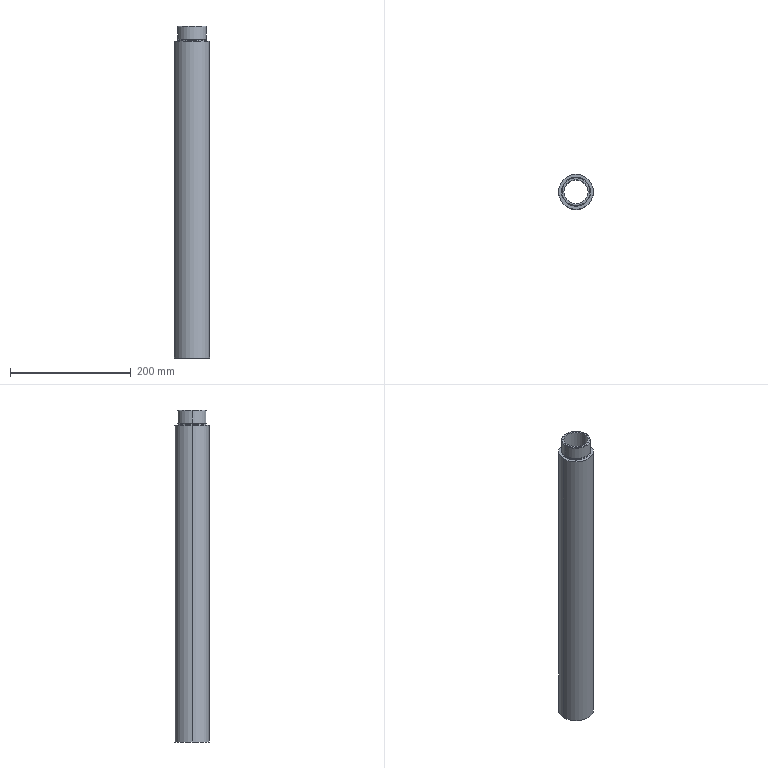Part | SolidWorks | features ICE 3, Chamfer 1, Extrusion 1, Fillet 1 | 1 solid | 18 faces | box 58 x 58 x 550 mm | volume 740682 mm3 | cylinder 8 | torus 4 | plane 4 | cone 2 | commonest cylinder face diameters 40 x2 45.8 x2 48 x2 58 x2
STEP:
#1=CARTESIAN_POINT('',(-23.9,0.,528.));
#2=VERTEX_POINT('',#1);
#3=CARTESIAN_POINT('',(23.9,0.,528.));
#4=VERTEX_POINT('',#3);
#5=CARTESIAN_POINT('',(0.,0.,528.));
#6=DIRECTION('',(0.,0.,1.));
#7=DIRECTION('',(1.,0.,0.));
#8=AXIS2_PLACEMENT_3D('',#5,#6,#7);
#9=CIRCLE('',#8,23.9);
#10=EDGE_CURVE('',#2,#4,#9,.T.);
#11=ORIENTED_EDGE('',*,*,#10,.F.);
#12=CARTESIAN_POINT('',(-22.9,0.,527.));
#13=VERTEX_POINT('',#12);
#14=CARTESIAN_POINT('',(-23.9,0.,527.));
#15=DIRECTION('',(0.,1.,0.));
#16=DIRECTION('',(-1.,0.,0.));
#17=AXIS2_PLACEMENT_3D('',#14,#15,#16);
#18=CIRCLE('',#17,1.);
#19=EDGE_CURVE('',#2,#13,#18,.T.);
#20=ORIENTED_EDGE('',*,*,#19,.T.);
#21=CARTESIAN_POINT('',(22.9,0.,527.));
#22=VERTEX_POINT('',#21);
#23=CARTESIAN_POINT('',(0.,0.,527.));
#24=DIRECTION('',(0.,0.,-1.));
#25=DIRECTION('',(1.,0.,0.));
#26=AXIS2_PLACEMENT_3D('',#23,#24,#25);
#27=CIRCLE('',#26,22.9);
#28=EDGE_CURVE('',#22,#13,#27,.T.);
#29=ORIENTED_EDGE('',*,*,#28,.F.);
#30=CARTESIAN_POINT('',(23.9,0.,527.));
#31=DIRECTION('',(0.,-1.,0.));
#32=DIRECTION('',(0.,0.,-1.));
#33=AXIS2_PLACEMENT_3D('',#30,#31,#32);
#34=CIRCLE('',#33,1.);
#35=EDGE_CURVE('',#4,#22,#34,.T.);
#36=ORIENTED_EDGE('',*,*,#35,.F.);
#37=EDGE_LOOP('',(#11,#20,#29,#36));
#38=FACE_OUTER_BOUND('',#37,.T.);
#39=CARTESIAN_POINT('',(0.,0.,527.));
#40=DIRECTION('',(0.,0.,1.));
#41=DIRECTION('',(1.,0.,0.));
#42=AXIS2_PLACEMENT_3D('',#39,#40,#41);
#43=TOROIDAL_SURFACE('',#42,23.9,1.);
#44=ADVANCED_FACE('',(#38),#43,.F.);
#45=CARTESIAN_POINT('',(-22.9,0.,526.));
#46=VERTEX_POINT('',#45);
#47=CARTESIAN_POINT('',(22.9,0.,526.));
#48=VERTEX_POINT('',#47);
#49=CARTESIAN_POINT('',(0.,0.,526.));
#50=DIRECTION('',(0.,0.,1.));
#51=DIRECTION('',(1.,0.,0.));
#52=AXIS2_PLACEMENT_3D('',#49,#50,#51);
#53=CIRCLE('',#52,22.9);
#54=EDGE_CURVE('',#46,#48,#53,.T.);
#55=ORIENTED_EDGE('',*,*,#54,.F.);
#56=CARTESIAN_POINT('',(-23.9,0.,525.));
#57=VERTEX_POINT('',#56);
#58=CARTESIAN_POINT('',(-23.9,0.,526.));
#59=DIRECTION('',(0.,1.,0.));
#60=DIRECTION('',(-1.,0.,0.));
#61=AXIS2_PLACEMENT_3D('',#58,#59,#60);
#62=CIRCLE('',#61,1.);
#63=EDGE_CURVE('',#46,#57,#62,.T.);
#64=ORIENTED_EDGE('',*,*,#63,.T.);
#65=CARTESIAN_POINT('',(23.9,0.,525.));
#66=VERTEX_POINT('',#65);
#67=CARTESIAN_POINT('',(0.,0.,525.));
#68=DIRECTION('',(0.,0.,-1.));
#69=DIRECTION('',(1.,0.,0.));
#70=AXIS2_PLACEMENT_3D('',#67,#68,#69);
#71=CIRCLE('',#70,23.9);
#72=EDGE_CURVE('',#66,#57,#71,.T.);
#73=ORIENTED_EDGE('',*,*,#72,.F.);
#74=CARTESIAN_POINT('',(23.9,0.,526.));
#75=DIRECTION('',(0.,-1.,0.));
#76=DIRECTION('',(0.,0.,-1.));
#77=AXIS2_PLACEMENT_3D('',#74,#75,#76);
#78=CIRCLE('',#77,1.);
#79=EDGE_CURVE('',#48,#66,#78,.T.);
#80=ORIENTED_EDGE('',*,*,#79,.F.);
#81=EDGE_LOOP('',(#55,#64,#73,#80));
#82=FACE_OUTER_BOUND('',#81,.T.);
#83=CARTESIAN_POINT('',(0.,0.,526.));
#84=DIRECTION('',(0.,0.,1.));
#85=DIRECTION('',(1.,0.,0.));
#86=AXIS2_PLACEMENT_3D('',#83,#84,#85);
#87=TOROIDAL_SURFACE('',#86,23.9,1.);
#88=ADVANCED_FACE('',(#82),#87,.F.);
#89=CARTESIAN_POINT('',(0.,0.,527.));
#90=DIRECTION('',(0.,0.,-1.));
#91=DIRECTION('',(1.,0.,0.));
#92=AXIS2_PLACEMENT_3D('',#89,#90,#91);
#93=CIRCLE('',#92,22.9);
#94=EDGE_CURVE('',#13,#22,#93,.T.);
#95=ORIENTED_EDGE('',*,*,#94,.T.);
#96=CARTESIAN_POINT('',(22.9,0.,528.));
#97=DIRECTION('',(0.,0.,-1.));
#98=VECTOR('',#97,1000.);
#99=LINE('',#96,#98);
#100=EDGE_CURVE('',#22,#48,#99,.T.);
#101=ORIENTED_EDGE('',*,*,#100,.T.);
#102=CARTESIAN_POINT('',(0.,0.,526.));
#103=DIRECTION('',(0.,0.,1.));
#104=DIRECTION('',(1.,0.,0.));
#105=AXIS2_PLACEMENT_3D('',#102,#103,#104);
#106=CIRCLE('',#105,22.9);
#107=EDGE_CURVE('',#48,#46,#106,.T.);
#108=ORIENTED_EDGE('',*,*,#107,.T.);
#109=CARTESIAN_POINT('',(-22.9,0.,528.));
#110=DIRECTION('',(0.,0.,-1.));
#111=VECTOR('',#110,1000.);
#112=LINE('',#109,#111);
#113=EDGE_CURVE('',#13,#46,#112,.T.);
#114=ORIENTED_EDGE('',*,*,#113,.F.);
#115=EDGE_LOOP('',(#95,#101,#108,#114));
#116=FACE_OUTER_BOUND('',#115,.T.);
#117=CARTESIAN_POINT('',(0.,0.,528.));
#118=DIRECTION('',(0.,0.,-1.));
#119=DIRECTION('',(-1.,0.,0.));
#120=AXIS2_PLACEMENT_3D('',#117,#118,#119);
#121=CYLINDRICAL_SURFACE('',#120,22.9);
#122=ADVANCED_FACE('',(#116),#121,.T.);
#123=CARTESIAN_POINT('',(23.,0.,550.));
#124=VERTEX_POINT('',#123);
#125=CARTESIAN_POINT('',(-23.,0.,550.));
#126=VERTEX_POINT('',#125);
#127=CARTESIAN_POINT('',(0.,0.,550.));
#128=DIRECTION('',(0.,0.,1.));
#129=DIRECTION('',(1.,0.,0.));
#130=AXIS2_PLACEMENT_3D('',#127,#128,#129);
#131=CIRCLE('',#130,23.);
#132=EDGE_CURVE('',#124,#126,#131,.T.);
#133=ORIENTED_EDGE('',*,*,#132,.F.);
#134=CARTESIAN_POINT('',(24.,0.,549.));
#135=VERTEX_POINT('',#134);
#136=CARTESIAN_POINT('',(23.,0.,550.));
#137=DIRECTION('',(0.7071,0.,-0.7071));
#138=VECTOR('',#137,1000.);
#139=LINE('',#136,#138);
#140=EDGE_CURVE('',#124,#135,#139,.T.);
#141=ORIENTED_EDGE('',*,*,#140,.T.);
#142=CARTESIAN_POINT('',(-24.,0.,549.));
#143=VERTEX_POINT('',#142);
#144=CARTESIAN_POINT('',(0.,0.,549.));
#145=DIRECTION('',(0.,0.,-1.));
#146=DIRECTION('',(1.,0.,0.));
#147=AXIS2_PLACEMENT_3D('',#144,#145,#146);
#148=CIRCLE('',#147,24.);
#149=EDGE_CURVE('',#143,#135,#148,.T.);
#150=ORIENTED_EDGE('',*,*,#149,.F.);
#151=CARTESIAN_POINT('',(-23.,0.,550.));
#152=DIRECTION('',(-0.7071,0.,-0.7071));
#153=VECTOR('',#152,1000.);
#154=LINE('',#151,#153);
#155=EDGE_CURVE('',#126,#143,#154,.T.);
#156=ORIENTED_EDGE('',*,*,#155,.F.);
#157=EDGE_LOOP('',(#133,#141,#150,#156));
#158=FACE_OUTER_BOUND('',#157,.T.);
#159=CARTESIAN_POINT('',(0.,0.,550.));
#160=DIRECTION('',(0.,0.,-1.));
#161=DIRECTION('',(-1.,0.,0.));
#162=AXIS2_PLACEMENT_3D('',#159,#160,#161);
#163=CONICAL_SURFACE('',#162,23.,0.7854);
#164=ADVANCED_FACE('',(#158),#163,.T.);
#165=CARTESIAN_POINT('',(-20.,0.,0.));
#166=VERTEX_POINT('',#165);
#167=CARTESIAN_POINT('',(20.,0.,0.));
#168=VERTEX_POINT('',#167);
#169=CARTESIAN_POINT('',(0.,0.,0.));
#170=DIRECTION('',(0.,0.,1.));
#171=DIRECTION('',(1.,0.,0.));
#172=AXIS2_PLACEMENT_3D('',#169,#170,#171);
#173=CIRCLE('',#172,20.);
#174=EDGE_CURVE('',#166,#168,#173,.T.);
#175=ORIENTED_EDGE('',*,*,#174,.F.);
#176=CARTESIAN_POINT('',(-20.,0.,550.));
#177=VERTEX_POINT('',#176);
#178=CARTESIAN_POINT('',(-20.,0.,0.));
#179=DIRECTION('',(0.,0.,1.));
#180=VECTOR('',#179,1000.);
#181=LINE('',#178,#180);
#182=EDGE_CURVE('',#166,#177,#181,.T.);
#183=ORIENTED_EDGE('',*,*,#182,.T.);
#184=CARTESIAN_POINT('',(20.,0.,550.));
#185=VERTEX_POINT('',#184);
#186=CARTESIAN_POINT('',(0.,0.,550.));
#187=DIRECTION('',(0.,0.,1.));
#188=DIRECTION('',(1.,0.,0.));
#189=AXIS2_PLACEMENT_3D('',#186,#187,#188);
#190=CIRCLE('',#189,20.);
#191=EDGE_CURVE('',#177,#185,#190,.T.);
#192=ORIENTED_EDGE('',*,*,#191,.T.);
#193=CARTESIAN_POINT('',(20.,0.,0.));
#194=DIRECTION('',(0.,0.,1.));
#195=VECTOR('',#194,1000.);
#196=LINE('',#193,#195);
#197=EDGE_CURVE('',#168,#185,#196,.T.);
#198=ORIENTED_EDGE('',*,*,#197,.F.);
#199=EDGE_LOOP('',(#175,#183,#192,#198));
#200=FACE_OUTER_BOUND('',#199,.T.);
#201=CARTESIAN_POINT('',(0.,0.,0.));
#202=DIRECTION('',(0.,0.,1.));
#203=DIRECTION('',(1.,0.,0.));
#204=AXIS2_PLACEMENT_3D('',#201,#202,#203);
#205=CYLINDRICAL_SURFACE('',#204,20.);
#206=ADVANCED_FACE('',(#200),#205,.F.);
#207=CARTESIAN_POINT('',(24.,0.,528.));
#208=VERTEX_POINT('',#207);
#209=CARTESIAN_POINT('',(-24.,0.,528.));
#210=VERTEX_POINT('',#209);
#211=CARTESIAN_POINT('',(0.,0.,528.));
#212=DIRECTION('',(0.,0.,1.));
#213=DIRECTION('',(1.,0.,0.));
#214=AXIS2_PLACEMENT_3D('',#211,#212,#213);
#215=CIRCLE('',#214,24.);
#216=EDGE_CURVE('',#208,#210,#215,.T.);
#217=ORIENTED_EDGE('',*,*,#216,.T.);
#218=CARTESIAN_POINT('',(-24.,0.,525.));
#219=DIRECTION('',(0.,0.,1.));
#220=VECTOR('',#219,1000.);
#221=LINE('',#218,#220);
#222=EDGE_CURVE('',#210,#143,#221,.T.);
#223=ORIENTED_EDGE('',*,*,#222,.T.);
#224=ORIENTED_EDGE('',*,*,#149,.T.);
#225=CARTESIAN_POINT('',(24.,0.,525.));
#226=DIRECTION('',(0.,0.,1.));
#227=VECTOR('',#226,1000.);
#228=LINE('',#225,#227);
#229=EDGE_CURVE('',#208,#135,#228,.T.);
#230=ORIENTED_EDGE('',*,*,#229,.F.);
#231=EDGE_LOOP('',(#217,#223,#224,#230));
#232=FACE_OUTER_BOUND('',#231,.T.);
#233=CARTESIAN_POINT('',(0.,0.,525.));
#234=DIRECTION('',(0.,0.,1.));
#235=DIRECTION('',(1.,0.,0.));
#236=AXIS2_PLACEMENT_3D('',#233,#234,#235);
#237=CYLINDRICAL_SURFACE('',#236,24.);
#238=ADVANCED_FACE('',(#232),#237,.T.);
#239=CARTESIAN_POINT('',(29.,0.,525.));
#240=VERTEX_POINT('',#239);
#241=CARTESIAN_POINT('',(-29.,0.,525.));
#242=VERTEX_POINT('',#241);
#243=CARTESIAN_POINT('',(0.,0.,525.));
#244=DIRECTION('',(0.,0.,1.));
#245=DIRECTION('',(1.,0.,0.));
#246=AXIS2_PLACEMENT_3D('',#243,#244,#245);
#247=CIRCLE('',#246,29.);
#248=EDGE_CURVE('',#240,#242,#247,.T.);
#249=ORIENTED_EDGE('',*,*,#248,.F.);
#250=CARTESIAN_POINT('',(29.,0.,0.));
#251=VERTEX_POINT('',#250);
#252=CARTESIAN_POINT('',(29.,0.,550.));
#253=DIRECTION('',(0.,0.,-1.));
#254=VECTOR('',#253,1000.);
#255=LINE('',#252,#254);
#256=EDGE_CURVE('',#240,#251,#255,.T.);
#257=ORIENTED_EDGE('',*,*,#256,.T.);
#258=CARTESIAN_POINT('',(-29.,0.,0.));
#259=VERTEX_POINT('',#258);
#260=CARTESIAN_POINT('',(0.,0.,0.));
#261=DIRECTION('',(0.,0.,1.));
#262=DIRECTION('',(1.,0.,0.));
#263=AXIS2_PLACEMENT_3D('',#260,#261,#262);
#264=CIRCLE('',#263,29.);
#265=EDGE_CURVE('',#251,#259,#264,.T.);
#266=ORIENTED_EDGE('',*,*,#265,.T.);
#267=CARTESIAN_POINT('',(-29.,0.,550.));
#268=DIRECTION('',(0.,0.,-1.));
#269=VECTOR('',#268,1000.);
#270=LINE('',#267,#269);
#271=EDGE_CURVE('',#242,#259,#270,.T.);
#272=ORIENTED_EDGE('',*,*,#271,.F.);
#273=EDGE_LOOP('',(#249,#257,#266,#272));
#274=FACE_OUTER_BOUND('',#273,.T.);
#275=CARTESIAN_POINT('',(0.,0.,550.));
#276=DIRECTION('',(0.,0.,-1.));
#277=DIRECTION('',(-1.,0.,0.));
#278=AXIS2_PLACEMENT_3D('',#275,#276,#277);
#279=CYLINDRICAL_SURFACE('',#278,29.);
#280=ADVANCED_FACE('',(#274),#279,.T.);
#281=ORIENTED_EDGE('',*,*,#256,.F.);
#282=CARTESIAN_POINT('',(0.,0.,525.));
#283=DIRECTION('',(0.,0.,1.));
#284=DIRECTION('',(1.,0.,0.));
#285=AXIS2_PLACEMENT_3D('',#282,#283,#284);
#286=CIRCLE('',#285,29.);
#287=EDGE_CURVE('',#242,#240,#286,.T.);
#288=ORIENTED_EDGE('',*,*,#287,.F.);
#289=ORIENTED_EDGE('',*,*,#271,.T.);
#290=CARTESIAN_POINT('',(0.,0.,0.));
#291=DIRECTION('',(0.,0.,1.));
#292=DIRECTION('',(1.,0.,0.));
#293=AXIS2_PLACEMENT_3D('',#290,#291,#292);
#294=CIRCLE('',#293,29.);
#295=EDGE_CURVE('',#259,#251,#294,.T.);
#296=ORIENTED_EDGE('',*,*,#295,.T.);
#297=EDGE_LOOP('',(#281,#288,#289,#296));
#298=FACE_OUTER_BOUND('',#297,.T.);
#299=CARTESIAN_POINT('',(0.,0.,550.));
#300=DIRECTION('',(0.,0.,-1.));
#301=DIRECTION('',(-1.,0.,0.));
#302=AXIS2_PLACEMENT_3D('',#299,#300,#301);
#303=CYLINDRICAL_SURFACE('',#302,29.);
#304=ADVANCED_FACE('',(#298),#303,.T.);
#305=CARTESIAN_POINT('',(0.,0.,0.));
#306=DIRECTION('',(0.,0.,1.));
#307=DIRECTION('',(1.,0.,0.));
#308=AXIS2_PLACEMENT_3D('',#305,#306,#307);
#309=CIRCLE('',#308,20.);
#310=EDGE_CURVE('',#168,#166,#309,.T.);
#311=ORIENTED_EDGE('',*,*,#310,.T.);
#312=ORIENTED_EDGE('',*,*,#174,.T.);
#313=EDGE_LOOP('',(#311,#312));
#314=FACE_BOUND('',#313,.T.);
#315=ORIENTED_EDGE('',*,*,#295,.F.);
#316=ORIENTED_EDGE('',*,*,#265,.F.);
#317=EDGE_LOOP('',(#315,#316));
#318=FACE_OUTER_BOUND('',#317,.T.);
#319=CARTESIAN_POINT('',(0.,0.,0.));
#320=DIRECTION('',(0.,0.,1.));
#321=DIRECTION('',(1.,0.,0.));
#322=AXIS2_PLACEMENT_3D('',#319,#320,#321);
#323=PLANE('',#322);
#324=ADVANCED_FACE('',(#314,#318),#323,.F.);
#325=ORIENTED_EDGE('',*,*,#72,.T.);
#326=CARTESIAN_POINT('',(0.,0.,525.));
#327=DIRECTION('',(0.,0.,-1.));
#328=DIRECTION('',(1.,0.,0.));
#329=AXIS2_PLACEMENT_3D('',#326,#327,#328);
#330=CIRCLE('',#329,23.9);
#331=EDGE_CURVE('',#57,#66,#330,.T.);
#332=ORIENTED_EDGE('',*,*,#331,.T.);
#333=EDGE_LOOP('',(#325,#332));
#334=FACE_BOUND('',#333,.T.);
#335=ORIENTED_EDGE('',*,*,#287,.T.);
#336=ORIENTED_EDGE('',*,*,#248,.T.);
#337=EDGE_LOOP('',(#335,#336));
#338=FACE_OUTER_BOUND('',#337,.T.);
#339=CARTESIAN_POINT('',(0.,0.,525.));
#340=DIRECTION('',(0.,0.,1.));
#341=DIRECTION('',(1.,0.,0.));
#342=AXIS2_PLACEMENT_3D('',#339,#340,#341);
#343=PLANE('',#342);
#344=ADVANCED_FACE('',(#334,#338),#343,.T.);
#345=ORIENTED_EDGE('',*,*,#222,.F.);
#346=CARTESIAN_POINT('',(0.,0.,528.));
#347=DIRECTION('',(0.,0.,1.));
#348=DIRECTION('',(1.,0.,0.));
#349=AXIS2_PLACEMENT_3D('',#346,#347,#348);
#350=CIRCLE('',#349,24.);
#351=EDGE_CURVE('',#210,#208,#350,.T.);
#352=ORIENTED_EDGE('',*,*,#351,.T.);
#353=ORIENTED_EDGE('',*,*,#229,.T.);
#354=CARTESIAN_POINT('',(0.,0.,549.));
#355=DIRECTION('',(0.,0.,-1.));
#356=DIRECTION('',(1.,0.,0.));
#357=AXIS2_PLACEMENT_3D('',#354,#355,#356);
#358=CIRCLE('',#357,24.);
#359=EDGE_CURVE('',#135,#143,#358,.T.);
#360=ORIENTED_EDGE('',*,*,#359,.T.);
#361=EDGE_LOOP('',(#345,#352,#353,#360));
#362=FACE_OUTER_BOUND('',#361,.T.);
#363=CARTESIAN_POINT('',(0.,0.,525.));
#364=DIRECTION('',(0.,0.,1.));
#365=DIRECTION('',(1.,0.,0.));
#366=AXIS2_PLACEMENT_3D('',#363,#364,#365);
#367=CYLINDRICAL_SURFACE('',#366,24.);
#368=ADVANCED_FACE('',(#362),#367,.T.);
#369=CARTESIAN_POINT('',(0.,0.,550.));
#370=DIRECTION('',(0.,0.,1.));
#371=DIRECTION('',(1.,0.,0.));
#372=AXIS2_PLACEMENT_3D('',#369,#370,#371);
#373=CIRCLE('',#372,23.);
#374=EDGE_CURVE('',#126,#124,#373,.T.);
#375=ORIENTED_EDGE('',*,*,#374,.T.);
#376=ORIENTED_EDGE('',*,*,#132,.T.);
#377=EDGE_LOOP('',(#375,#376));
#378=FACE_OUTER_BOUND('',#377,.T.);
#379=CARTESIAN_POINT('',(0.,0.,550.));
#380=DIRECTION('',(0.,0.,1.));
#381=DIRECTION('',(1.,0.,0.));
#382=AXIS2_PLACEMENT_3D('',#379,#380,#381);
#383=CIRCLE('',#382,20.);
#384=EDGE_CURVE('',#185,#177,#383,.T.);
#385=ORIENTED_EDGE('',*,*,#384,.F.);
#386=ORIENTED_EDGE('',*,*,#191,.F.);
#387=EDGE_LOOP('',(#385,#386));
#388=FACE_BOUND('',#387,.T.);
#389=CARTESIAN_POINT('',(0.,0.,550.));
#390=DIRECTION('',(0.,0.,1.));
#391=DIRECTION('',(1.,0.,0.));
#392=AXIS2_PLACEMENT_3D('',#389,#390,#391);
#393=PLANE('',#392);
#394=ADVANCED_FACE('',(#378,#388),#393,.T.);
#395=ORIENTED_EDGE('',*,*,#182,.F.);
#396=ORIENTED_EDGE('',*,*,#310,.F.);
#397=ORIENTED_EDGE('',*,*,#197,.T.);
#398=ORIENTED_EDGE('',*,*,#384,.T.);
#399=EDGE_LOOP('',(#395,#396,#397,#398));
#400=FACE_OUTER_BOUND('',#399,.T.);
#401=CARTESIAN_POINT('',(0.,0.,0.));
#402=DIRECTION('',(0.,0.,1.));
#403=DIRECTION('',(1.,0.,0.));
#404=AXIS2_PLACEMENT_3D('',#401,#402,#403);
#405=CYLINDRICAL_SURFACE('',#404,20.);
#406=ADVANCED_FACE('',(#400),#405,.F.);
#407=ORIENTED_EDGE('',*,*,#140,.F.);
#408=ORIENTED_EDGE('',*,*,#374,.F.);
#409=ORIENTED_EDGE('',*,*,#155,.T.);
#410=ORIENTED_EDGE('',*,*,#359,.F.);
#411=EDGE_LOOP('',(#407,#408,#409,#410));
#412=FACE_OUTER_BOUND('',#411,.T.);
#413=CARTESIAN_POINT('',(0.,0.,550.));
#414=DIRECTION('',(0.,0.,-1.));
#415=DIRECTION('',(-1.,0.,0.));
#416=AXIS2_PLACEMENT_3D('',#413,#414,#415);
#417=CONICAL_SURFACE('',#416,23.,0.7854);
#418=ADVANCED_FACE('',(#412),#417,.T.);
#419=CARTESIAN_POINT('',(0.,0.,528.));
#420=DIRECTION('',(0.,0.,1.));
#421=DIRECTION('',(1.,0.,0.));
#422=AXIS2_PLACEMENT_3D('',#419,#420,#421);
#423=CIRCLE('',#422,23.9);
#424=EDGE_CURVE('',#4,#2,#423,.T.);
#425=ORIENTED_EDGE('',*,*,#424,.T.);
#426=ORIENTED_EDGE('',*,*,#10,.T.);
#427=EDGE_LOOP('',(#425,#426));
#428=FACE_BOUND('',#427,.T.);
#429=ORIENTED_EDGE('',*,*,#216,.F.);
#430=ORIENTED_EDGE('',*,*,#351,.F.);
#431=EDGE_LOOP('',(#429,#430));
#432=FACE_OUTER_BOUND('',#431,.T.);
#433=CARTESIAN_POINT('',(0.,0.,528.));
#434=DIRECTION('',(0.,0.,1.));
#435=DIRECTION('',(1.,0.,0.));
#436=AXIS2_PLACEMENT_3D('',#433,#434,#435);
#437=PLANE('',#436);
#438=ADVANCED_FACE('',(#428,#432),#437,.F.);
#439=ORIENTED_EDGE('',*,*,#100,.F.);
#440=ORIENTED_EDGE('',*,*,#28,.T.);
#441=ORIENTED_EDGE('',*,*,#113,.T.);
#442=ORIENTED_EDGE('',*,*,#54,.T.);
#443=EDGE_LOOP('',(#439,#440,#441,#442));
#444=FACE_OUTER_BOUND('',#443,.T.);
#445=CARTESIAN_POINT('',(0.,0.,528.));
#446=DIRECTION('',(0.,0.,-1.));
#447=DIRECTION('',(-1.,0.,0.));
#448=AXIS2_PLACEMENT_3D('',#445,#446,#447);
#449=CYLINDRICAL_SURFACE('',#448,22.9);
#450=ADVANCED_FACE('',(#444),#449,.T.);
#451=ORIENTED_EDGE('',*,*,#63,.F.);
#452=ORIENTED_EDGE('',*,*,#107,.F.);
#453=ORIENTED_EDGE('',*,*,#79,.T.);
#454=ORIENTED_EDGE('',*,*,#331,.F.);
#455=EDGE_LOOP('',(#451,#452,#453,#454));
#456=FACE_OUTER_BOUND('',#455,.T.);
#457=CARTESIAN_POINT('',(0.,0.,526.));
#458=DIRECTION('',(0.,0.,1.));
#459=DIRECTION('',(1.,0.,0.));
#460=AXIS2_PLACEMENT_3D('',#457,#458,#459);
#461=TOROIDAL_SURFACE('',#460,23.9,1.);
#462=ADVANCED_FACE('',(#456),#461,.F.);
#463=ORIENTED_EDGE('',*,*,#19,.F.);
#464=ORIENTED_EDGE('',*,*,#424,.F.);
#465=ORIENTED_EDGE('',*,*,#35,.T.);
#466=ORIENTED_EDGE('',*,*,#94,.F.);
#467=EDGE_LOOP('',(#463,#464,#465,#466));
#468=FACE_OUTER_BOUND('',#467,.T.);
#469=CARTESIAN_POINT('',(0.,0.,527.));
#470=DIRECTION('',(0.,0.,1.));
#471=DIRECTION('',(1.,0.,0.));
#472=AXIS2_PLACEMENT_3D('',#469,#470,#471);
#473=TOROIDAL_SURFACE('',#472,23.9,1.);
#474=ADVANCED_FACE('',(#468),#473,.F.);
#475=CLOSED_SHELL('',(#44,#88,#122,#164,#206,#238,#280,#304,#324,#344,#368,#394,#406,#418,#438,#450,#462,#474));
#476=MANIFOLD_SOLID_BREP('',#475);
#477=CARTESIAN_POINT('',(0.,0.,0.));
#478=DIRECTION('',(0.,0.,1.));
#479=DIRECTION('',(1.,0.,0.));
#480=AXIS2_PLACEMENT_3D('',#477,#478,#479);
#481=(LENGTH_UNIT()NAMED_UNIT(*)SI_UNIT(.MILLI.,.METRE.));
#482=UNCERTAINTY_MEASURE_WITH_UNIT(LENGTH_MEASURE(0.00001),#481,'','');
#483=(NAMED_UNIT(*)PLANE_ANGLE_UNIT()SI_UNIT($,.RADIAN.));
#484=(NAMED_UNIT(*)SI_UNIT($,.STERADIAN.)SOLID_ANGLE_UNIT());
#485=(GEOMETRIC_REPRESENTATION_CONTEXT(3)GLOBAL_UNCERTAINTY_ASSIGNED_CONTEXT((#482))GLOBAL_UNIT_ASSIGNED_CONTEXT((#481,#483,#484))REPRESENTATION_CONTEXT('',''));
#486=ADVANCED_BREP_SHAPE_REPRESENTATION('',(#476,#480),#485);